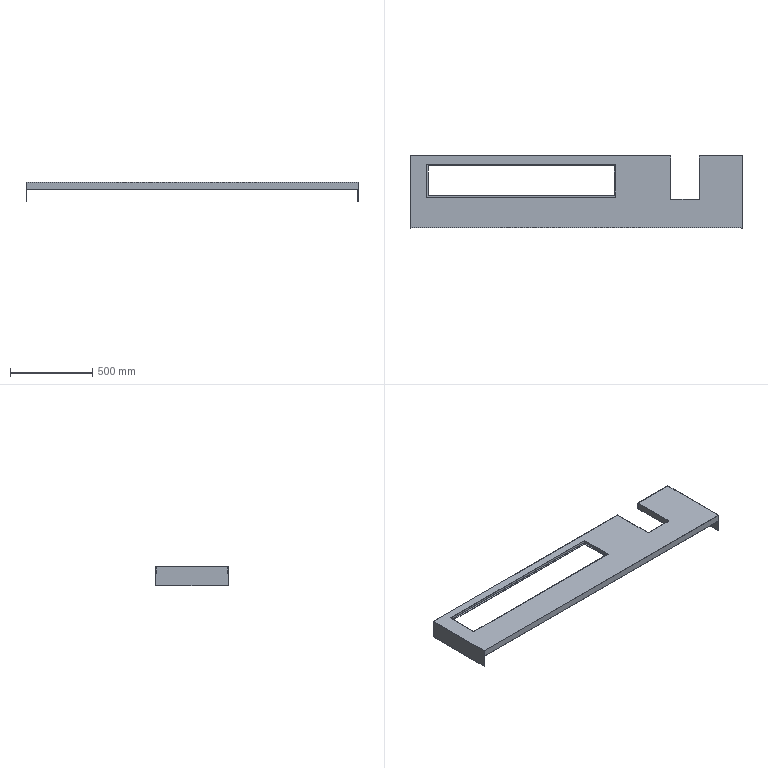Part | SolidWorks | features ICE 7, Extrusion 1 | 1 solid | 36 faces | box 2015 x 437 x 116 mm | volume 1908304 mm3 | plane 36
STEP:
#1=CARTESIAN_POINT('',(100.,387.,-13.));
#2=VERTEX_POINT('',#1);
#3=CARTESIAN_POINT('',(100.,187.,-13.));
#4=VERTEX_POINT('',#3);
#5=CARTESIAN_POINT('',(100.,387.,-13.));
#6=DIRECTION('',(0.,-1.,0.));
#7=VECTOR('',#6,1000.);
#8=LINE('',#5,#7);
#9=EDGE_CURVE('',#2,#4,#8,.T.);
#10=ORIENTED_EDGE('',*,*,#9,.F.);
#11=CARTESIAN_POINT('',(100.,387.,2.));
#12=VERTEX_POINT('',#11);
#13=CARTESIAN_POINT('',(100.,387.,-8.));
#14=DIRECTION('',(0.,0.,1.));
#15=VECTOR('',#14,1000.);
#16=LINE('',#13,#15);
#17=EDGE_CURVE('',#2,#12,#16,.T.);
#18=ORIENTED_EDGE('',*,*,#17,.T.);
#19=CARTESIAN_POINT('',(100.,187.,2.));
#20=VERTEX_POINT('',#19);
#21=CARTESIAN_POINT('',(100.,387.,2.));
#22=DIRECTION('',(0.,-1.,0.));
#23=VECTOR('',#22,1000.);
#24=LINE('',#21,#23);
#25=EDGE_CURVE('',#12,#20,#24,.T.);
#26=ORIENTED_EDGE('',*,*,#25,.T.);
#27=CARTESIAN_POINT('',(100.,187.,-8.));
#28=DIRECTION('',(0.,0.,1.));
#29=VECTOR('',#28,1000.);
#30=LINE('',#27,#29);
#31=EDGE_CURVE('',#4,#20,#30,.T.);
#32=ORIENTED_EDGE('',*,*,#31,.F.);
#33=EDGE_LOOP('',(#10,#18,#26,#32));
#34=FACE_OUTER_BOUND('',#33,.T.);
#35=CARTESIAN_POINT('',(100.,387.,-8.));
#36=DIRECTION('',(-1.,0.,0.));
#37=DIRECTION('',(0.,-1.,0.));
#38=AXIS2_PLACEMENT_3D('',#35,#36,#37);
#39=PLANE('',#38);
#40=ADVANCED_FACE('',(#34),#39,.F.);
#41=CARTESIAN_POINT('',(1250.,387.,-13.));
#42=VERTEX_POINT('',#41);
#43=CARTESIAN_POINT('',(100.,387.,-13.));
#44=DIRECTION('',(-1.,0.,0.));
#45=VECTOR('',#44,1000.);
#46=LINE('',#43,#45);
#47=EDGE_CURVE('',#42,#2,#46,.T.);
#48=ORIENTED_EDGE('',*,*,#47,.F.);
#49=CARTESIAN_POINT('',(1250.,387.,2.));
#50=VERTEX_POINT('',#49);
#51=CARTESIAN_POINT('',(1250.,387.,-8.));
#52=DIRECTION('',(0.,0.,1.));
#53=VECTOR('',#52,1000.);
#54=LINE('',#51,#53);
#55=EDGE_CURVE('',#42,#50,#54,.T.);
#56=ORIENTED_EDGE('',*,*,#55,.T.);
#57=CARTESIAN_POINT('',(100.,387.,2.));
#58=DIRECTION('',(-1.,0.,0.));
#59=VECTOR('',#58,1000.);
#60=LINE('',#57,#59);
#61=EDGE_CURVE('',#50,#12,#60,.T.);
#62=ORIENTED_EDGE('',*,*,#61,.T.);
#63=ORIENTED_EDGE('',*,*,#17,.F.);
#64=EDGE_LOOP('',(#48,#56,#62,#63));
#65=FACE_OUTER_BOUND('',#64,.T.);
#66=CARTESIAN_POINT('',(100.,387.,-8.));
#67=DIRECTION('',(0.,1.,0.));
#68=DIRECTION('',(0.,0.,1.));
#69=AXIS2_PLACEMENT_3D('',#66,#67,#68);
#70=PLANE('',#69);
#71=ADVANCED_FACE('',(#65),#70,.F.);
#72=CARTESIAN_POINT('',(1250.,187.,-13.));
#73=VERTEX_POINT('',#72);
#74=CARTESIAN_POINT('',(1250.,387.,-13.));
#75=DIRECTION('',(0.,1.,0.));
#76=VECTOR('',#75,1000.);
#77=LINE('',#74,#76);
#78=EDGE_CURVE('',#73,#42,#77,.T.);
#79=ORIENTED_EDGE('',*,*,#78,.F.);
#80=CARTESIAN_POINT('',(1250.,187.,2.));
#81=VERTEX_POINT('',#80);
#82=CARTESIAN_POINT('',(1250.,187.,-8.));
#83=DIRECTION('',(0.,0.,1.));
#84=VECTOR('',#83,1000.);
#85=LINE('',#82,#84);
#86=EDGE_CURVE('',#73,#81,#85,.T.);
#87=ORIENTED_EDGE('',*,*,#86,.T.);
#88=CARTESIAN_POINT('',(1250.,387.,2.));
#89=DIRECTION('',(0.,1.,0.));
#90=VECTOR('',#89,1000.);
#91=LINE('',#88,#90);
#92=EDGE_CURVE('',#81,#50,#91,.T.);
#93=ORIENTED_EDGE('',*,*,#92,.T.);
#94=ORIENTED_EDGE('',*,*,#55,.F.);
#95=EDGE_LOOP('',(#79,#87,#93,#94));
#96=FACE_OUTER_BOUND('',#95,.T.);
#97=CARTESIAN_POINT('',(1250.,387.,-8.));
#98=DIRECTION('',(1.,0.,0.));
#99=DIRECTION('',(0.,0.,-1.));
#100=AXIS2_PLACEMENT_3D('',#97,#98,#99);
#101=PLANE('',#100);
#102=ADVANCED_FACE('',(#96),#101,.F.);
#103=CARTESIAN_POINT('',(100.,187.,-13.));
#104=DIRECTION('',(1.,0.,0.));
#105=VECTOR('',#104,1000.);
#106=LINE('',#103,#105);
#107=EDGE_CURVE('',#4,#73,#106,.T.);
#108=ORIENTED_EDGE('',*,*,#107,.F.);
#109=ORIENTED_EDGE('',*,*,#31,.T.);
#110=CARTESIAN_POINT('',(100.,187.,2.));
#111=DIRECTION('',(1.,0.,0.));
#112=VECTOR('',#111,1000.);
#113=LINE('',#110,#112);
#114=EDGE_CURVE('',#20,#81,#113,.T.);
#115=ORIENTED_EDGE('',*,*,#114,.T.);
#116=ORIENTED_EDGE('',*,*,#86,.F.);
#117=EDGE_LOOP('',(#108,#109,#115,#116));
#118=FACE_OUTER_BOUND('',#117,.T.);
#119=CARTESIAN_POINT('',(100.,187.,-8.));
#120=DIRECTION('',(0.,-1.,0.));
#121=DIRECTION('',(0.,0.,-1.));
#122=AXIS2_PLACEMENT_3D('',#119,#120,#121);
#123=PLANE('',#122);
#124=ADVANCED_FACE('',(#118),#123,.F.);
#125=CARTESIAN_POINT('',(2013.,2.,0.));
#126=VERTEX_POINT('',#125);
#127=CARTESIAN_POINT('',(2013.,435.,0.));
#128=VERTEX_POINT('',#127);
#129=CARTESIAN_POINT('',(2013.,0.,0.));
#130=DIRECTION('',(0.,1.,0.));
#131=VECTOR('',#130,1000.);
#132=LINE('',#129,#131);
#133=EDGE_CURVE('',#126,#128,#132,.T.);
#134=ORIENTED_EDGE('',*,*,#133,.F.);
#135=CARTESIAN_POINT('',(2.,2.,0.));
#136=VERTEX_POINT('',#135);
#137=CARTESIAN_POINT('',(0.,2.,0.));
#138=DIRECTION('',(-1.,0.,0.));
#139=VECTOR('',#138,1000.);
#140=LINE('',#137,#139);
#141=EDGE_CURVE('',#126,#136,#140,.T.);
#142=ORIENTED_EDGE('',*,*,#141,.T.);
#143=CARTESIAN_POINT('',(2.,435.,0.));
#144=VERTEX_POINT('',#143);
#145=CARTESIAN_POINT('',(2.,437.,0.));
#146=DIRECTION('',(0.,-1.,0.));
#147=VECTOR('',#146,1000.);
#148=LINE('',#145,#147);
#149=EDGE_CURVE('',#144,#136,#148,.T.);
#150=ORIENTED_EDGE('',*,*,#149,.F.);
#151=CARTESIAN_POINT('',(1580.,435.,0.));
#152=VERTEX_POINT('',#151);
#153=CARTESIAN_POINT('',(1580.,435.,0.));
#154=DIRECTION('',(-1.,0.,0.));
#155=VECTOR('',#154,1000.);
#156=LINE('',#153,#155);
#157=EDGE_CURVE('',#152,#144,#156,.T.);
#158=ORIENTED_EDGE('',*,*,#157,.F.);
#159=CARTESIAN_POINT('',(1580.,171.,0.));
#160=VERTEX_POINT('',#159);
#161=CARTESIAN_POINT('',(1580.,171.,0.));
#162=DIRECTION('',(0.,1.,0.));
#163=VECTOR('',#162,1000.);
#164=LINE('',#161,#163);
#165=EDGE_CURVE('',#160,#152,#164,.T.);
#166=ORIENTED_EDGE('',*,*,#165,.F.);
#167=CARTESIAN_POINT('',(1759.,171.,0.));
#168=VERTEX_POINT('',#167);
#169=CARTESIAN_POINT('',(1759.,171.,0.));
#170=DIRECTION('',(-1.,0.,0.));
#171=VECTOR('',#170,1000.);
#172=LINE('',#169,#171);
#173=EDGE_CURVE('',#168,#160,#172,.T.);
#174=ORIENTED_EDGE('',*,*,#173,.F.);
#175=CARTESIAN_POINT('',(1759.,435.,0.));
#176=VERTEX_POINT('',#175);
#177=CARTESIAN_POINT('',(1759.,435.,0.));
#178=DIRECTION('',(0.,-1.,0.));
#179=VECTOR('',#178,1000.);
#180=LINE('',#177,#179);
#181=EDGE_CURVE('',#176,#168,#180,.T.);
#182=ORIENTED_EDGE('',*,*,#181,.F.);
#183=CARTESIAN_POINT('',(2013.,435.,0.));
#184=DIRECTION('',(-1.,0.,0.));
#185=VECTOR('',#184,1000.);
#186=LINE('',#183,#185);
#187=EDGE_CURVE('',#128,#176,#186,.T.);
#188=ORIENTED_EDGE('',*,*,#187,.F.);
#189=EDGE_LOOP('',(#134,#142,#150,#158,#166,#174,#182,#188));
#190=FACE_OUTER_BOUND('',#189,.T.);
#191=CARTESIAN_POINT('',(1252.,389.,0.));
#192=VERTEX_POINT('',#191);
#193=CARTESIAN_POINT('',(1252.,185.,0.));
#194=VERTEX_POINT('',#193);
#195=CARTESIAN_POINT('',(1252.,389.,0.));
#196=DIRECTION('',(0.,-1.,0.));
#197=VECTOR('',#196,1000.);
#198=LINE('',#195,#197);
#199=EDGE_CURVE('',#192,#194,#198,.T.);
#200=ORIENTED_EDGE('',*,*,#199,.F.);
#201=CARTESIAN_POINT('',(98.,389.,0.));
#202=VERTEX_POINT('',#201);
#203=CARTESIAN_POINT('',(98.,389.,0.));
#204=DIRECTION('',(1.,0.,0.));
#205=VECTOR('',#204,1000.);
#206=LINE('',#203,#205);
#207=EDGE_CURVE('',#202,#192,#206,.T.);
#208=ORIENTED_EDGE('',*,*,#207,.F.);
#209=CARTESIAN_POINT('',(98.,185.,0.));
#210=VERTEX_POINT('',#209);
#211=CARTESIAN_POINT('',(98.,185.,0.));
#212=DIRECTION('',(0.,1.,0.));
#213=VECTOR('',#212,1000.);
#214=LINE('',#211,#213);
#215=EDGE_CURVE('',#210,#202,#214,.T.);
#216=ORIENTED_EDGE('',*,*,#215,.F.);
#217=CARTESIAN_POINT('',(1252.,185.,0.));
#218=DIRECTION('',(-1.,0.,0.));
#219=VECTOR('',#218,1000.);
#220=LINE('',#217,#219);
#221=EDGE_CURVE('',#194,#210,#220,.T.);
#222=ORIENTED_EDGE('',*,*,#221,.F.);
#223=EDGE_LOOP('',(#200,#208,#216,#222));
#224=FACE_BOUND('',#223,.T.);
#225=CARTESIAN_POINT('',(0.,437.,0.));
#226=DIRECTION('',(0.,0.,-1.));
#227=DIRECTION('',(-1.,0.,0.));
#228=AXIS2_PLACEMENT_3D('',#225,#226,#227);
#229=PLANE('',#228);
#230=ADVANCED_FACE('',(#190,#224),#229,.T.);
#231=CARTESIAN_POINT('',(2013.,0.,-114.));
#232=VERTEX_POINT('',#231);
#233=CARTESIAN_POINT('',(2013.,0.,-40.468));
#234=VERTEX_POINT('',#233);
#235=CARTESIAN_POINT('',(2013.,0.,-114.));
#236=DIRECTION('',(0.,0.,1.));
#237=VECTOR('',#236,1000.);
#238=LINE('',#235,#237);
#239=EDGE_CURVE('',#232,#234,#238,.T.);
#240=ORIENTED_EDGE('',*,*,#239,.T.);
#241=CARTESIAN_POINT('',(2013.,2.,-40.468));
#242=VERTEX_POINT('',#241);
#243=CARTESIAN_POINT('',(2013.,0.,-40.468));
#244=DIRECTION('',(0.,1.,0.));
#245=VECTOR('',#244,1000.);
#246=LINE('',#243,#245);
#247=EDGE_CURVE('',#234,#242,#246,.T.);
#248=ORIENTED_EDGE('',*,*,#247,.T.);
#249=CARTESIAN_POINT('',(2013.,2.,-114.));
#250=DIRECTION('',(0.,0.,-1.));
#251=VECTOR('',#250,1000.);
#252=LINE('',#249,#251);
#253=EDGE_CURVE('',#126,#242,#252,.T.);
#254=ORIENTED_EDGE('',*,*,#253,.F.);
#255=ORIENTED_EDGE('',*,*,#133,.T.);
#256=CARTESIAN_POINT('',(2013.,435.,-40.));
#257=VERTEX_POINT('',#256);
#258=CARTESIAN_POINT('',(2013.,435.,-40.));
#259=DIRECTION('',(0.,0.,1.));
#260=VECTOR('',#259,1000.);
#261=LINE('',#258,#260);
#262=EDGE_CURVE('',#257,#128,#261,.T.);
#263=ORIENTED_EDGE('',*,*,#262,.F.);
#264=CARTESIAN_POINT('',(2013.,437.,-40.));
#265=VERTEX_POINT('',#264);
#266=CARTESIAN_POINT('',(2013.,437.,-40.));
#267=DIRECTION('',(0.,-1.,0.));
#268=VECTOR('',#267,1000.);
#269=LINE('',#266,#268);
#270=EDGE_CURVE('',#265,#257,#269,.T.);
#271=ORIENTED_EDGE('',*,*,#270,.F.);
#272=CARTESIAN_POINT('',(2013.,437.,-114.));
#273=VERTEX_POINT('',#272);
#274=CARTESIAN_POINT('',(2013.,437.,-114.));
#275=DIRECTION('',(0.,0.,1.));
#276=VECTOR('',#275,1000.);
#277=LINE('',#274,#276);
#278=EDGE_CURVE('',#273,#265,#277,.T.);
#279=ORIENTED_EDGE('',*,*,#278,.F.);
#280=CARTESIAN_POINT('',(2013.,0.,-114.));
#281=DIRECTION('',(0.,1.,0.));
#282=VECTOR('',#281,1000.);
#283=LINE('',#280,#282);
#284=EDGE_CURVE('',#232,#273,#283,.T.);
#285=ORIENTED_EDGE('',*,*,#284,.F.);
#286=EDGE_LOOP('',(#240,#248,#254,#255,#263,#271,#279,#285));
#287=FACE_OUTER_BOUND('',#286,.T.);
#288=CARTESIAN_POINT('',(2013.,0.,-114.));
#289=DIRECTION('',(1.,0.,0.));
#290=DIRECTION('',(0.,0.,-1.));
#291=AXIS2_PLACEMENT_3D('',#288,#289,#290);
#292=PLANE('',#291);
#293=ADVANCED_FACE('',(#287),#292,.F.);
#294=CARTESIAN_POINT('',(2.,2.,-40.468));
#295=VERTEX_POINT('',#294);
#296=CARTESIAN_POINT('',(2.,2.,-114.));
#297=DIRECTION('',(0.,0.,1.));
#298=VECTOR('',#297,1000.);
#299=LINE('',#296,#298);
#300=EDGE_CURVE('',#295,#136,#299,.T.);
#301=ORIENTED_EDGE('',*,*,#300,.F.);
#302=CARTESIAN_POINT('',(2.,0.,-40.468));
#303=VERTEX_POINT('',#302);
#304=CARTESIAN_POINT('',(2.,437.,-40.468));
#305=DIRECTION('',(0.,-1.,0.));
#306=VECTOR('',#305,1000.);
#307=LINE('',#304,#306);
#308=EDGE_CURVE('',#295,#303,#307,.T.);
#309=ORIENTED_EDGE('',*,*,#308,.T.);
#310=CARTESIAN_POINT('',(2.,0.,-114.));
#311=VERTEX_POINT('',#310);
#312=CARTESIAN_POINT('',(2.,0.,-114.));
#313=DIRECTION('',(0.,0.,1.));
#314=VECTOR('',#313,1000.);
#315=LINE('',#312,#314);
#316=EDGE_CURVE('',#311,#303,#315,.T.);
#317=ORIENTED_EDGE('',*,*,#316,.F.);
#318=CARTESIAN_POINT('',(2.,437.,-114.));
#319=VERTEX_POINT('',#318);
#320=CARTESIAN_POINT('',(2.,437.,-114.));
#321=DIRECTION('',(0.,-1.,0.));
#322=VECTOR('',#321,1000.);
#323=LINE('',#320,#322);
#324=EDGE_CURVE('',#319,#311,#323,.T.);
#325=ORIENTED_EDGE('',*,*,#324,.F.);
#326=CARTESIAN_POINT('',(2.,437.,-40.));
#327=VERTEX_POINT('',#326);
#328=CARTESIAN_POINT('',(2.,437.,-114.));
#329=DIRECTION('',(0.,0.,1.));
#330=VECTOR('',#329,1000.);
#331=LINE('',#328,#330);
#332=EDGE_CURVE('',#319,#327,#331,.T.);
#333=ORIENTED_EDGE('',*,*,#332,.T.);
#334=CARTESIAN_POINT('',(2.,435.,-40.));
#335=VERTEX_POINT('',#334);
#336=CARTESIAN_POINT('',(2.,437.,-40.));
#337=DIRECTION('',(0.,1.,0.));
#338=VECTOR('',#337,1000.);
#339=LINE('',#336,#338);
#340=EDGE_CURVE('',#335,#327,#339,.T.);
#341=ORIENTED_EDGE('',*,*,#340,.F.);
#342=CARTESIAN_POINT('',(2.,435.,-40.));
#343=DIRECTION('',(0.,0.,1.));
#344=VECTOR('',#343,1000.);
#345=LINE('',#342,#344);
#346=EDGE_CURVE('',#335,#144,#345,.T.);
#347=ORIENTED_EDGE('',*,*,#346,.T.);
#348=ORIENTED_EDGE('',*,*,#149,.T.);
#349=EDGE_LOOP('',(#301,#309,#317,#325,#333,#341,#347,#348));
#350=FACE_OUTER_BOUND('',#349,.T.);
#351=CARTESIAN_POINT('',(2.,437.,-114.));
#352=DIRECTION('',(-1.,0.,0.));
#353=DIRECTION('',(0.,-1.,0.));
#354=AXIS2_PLACEMENT_3D('',#351,#352,#353);
#355=PLANE('',#354);
#356=ADVANCED_FACE('',(#350),#355,.F.);
#357=CARTESIAN_POINT('',(0.,0.,-114.));
#358=VERTEX_POINT('',#357);
#359=CARTESIAN_POINT('',(0.,437.,-114.));
#360=VERTEX_POINT('',#359);
#361=CARTESIAN_POINT('',(0.,437.,-114.));
#362=DIRECTION('',(0.,1.,0.));
#363=VECTOR('',#362,1000.);
#364=LINE('',#361,#363);
#365=EDGE_CURVE('',#358,#360,#364,.T.);
#366=ORIENTED_EDGE('',*,*,#365,.F.);
#367=CARTESIAN_POINT('',(0.,0.,2.));
#368=VERTEX_POINT('',#367);
#369=CARTESIAN_POINT('',(0.,0.,2.));
#370=DIRECTION('',(0.,0.,-1.));
#371=VECTOR('',#370,1000.);
#372=LINE('',#369,#371);
#373=EDGE_CURVE('',#368,#358,#372,.T.);
#374=ORIENTED_EDGE('',*,*,#373,.F.);
#375=CARTESIAN_POINT('',(0.,437.,2.));
#376=VERTEX_POINT('',#375);
#377=CARTESIAN_POINT('',(0.,0.,2.));
#378=DIRECTION('',(0.,-1.,0.));
#379=VECTOR('',#378,1000.);
#380=LINE('',#377,#379);
#381=EDGE_CURVE('',#376,#368,#380,.T.);
#382=ORIENTED_EDGE('',*,*,#381,.F.);
#383=CARTESIAN_POINT('',(0.,437.,2.));
#384=DIRECTION('',(0.,0.,-1.));
#385=VECTOR('',#384,1000.);
#386=LINE('',#383,#385);
#387=EDGE_CURVE('',#376,#360,#386,.T.);
#388=ORIENTED_EDGE('',*,*,#387,.T.);
#389=EDGE_LOOP('',(#366,#374,#382,#388));
#390=FACE_OUTER_BOUND('',#389,.T.);
#391=CARTESIAN_POINT('',(0.,0.,2.));
#392=DIRECTION('',(1.,0.,0.));
#393=DIRECTION('',(0.,0.,-1.));
#394=AXIS2_PLACEMENT_3D('',#391,#392,#393);
#395=PLANE('',#394);
#396=ADVANCED_FACE('',(#390),#395,.F.);
#397=CARTESIAN_POINT('',(0.,0.,-40.468));
#398=DIRECTION('',(1.,0.,0.));
#399=VECTOR('',#398,1000.);
#400=LINE('',#397,#399);
#401=EDGE_CURVE('',#303,#234,#400,.T.);
#402=ORIENTED_EDGE('',*,*,#401,.T.);
#403=ORIENTED_EDGE('',*,*,#239,.F.);
#404=CARTESIAN_POINT('',(2015.,0.,-114.));
#405=VERTEX_POINT('',#404);
#406=CARTESIAN_POINT('',(2015.,0.,-114.));
#407=DIRECTION('',(-1.,0.,0.));
#408=VECTOR('',#407,1000.);
#409=LINE('',#406,#408);
#410=EDGE_CURVE('',#405,#232,#409,.T.);
#411=ORIENTED_EDGE('',*,*,#410,.F.);
#412=CARTESIAN_POINT('',(2015.,0.,2.));
#413=VERTEX_POINT('',#412);
#414=CARTESIAN_POINT('',(2015.,0.,2.));
#415=DIRECTION('',(0.,0.,-1.));
#416=VECTOR('',#415,1000.);
#417=LINE('',#414,#416);
#418=EDGE_CURVE('',#413,#405,#417,.T.);
#419=ORIENTED_EDGE('',*,*,#418,.F.);
#420=CARTESIAN_POINT('',(0.,0.,2.));
#421=DIRECTION('',(1.,0.,0.));
#422=VECTOR('',#421,1000.);
#423=LINE('',#420,#422);
#424=EDGE_CURVE('',#368,#413,#423,.T.);
#425=ORIENTED_EDGE('',*,*,#424,.F.);
#426=ORIENTED_EDGE('',*,*,#373,.T.);
#427=CARTESIAN_POINT('',(0.,0.,-114.));
#428=DIRECTION('',(-1.,0.,0.));
#429=VECTOR('',#428,1000.);
#430=LINE('',#427,#429);
#431=EDGE_CURVE('',#311,#358,#430,.T.);
#432=ORIENTED_EDGE('',*,*,#431,.F.);
#433=ORIENTED_EDGE('',*,*,#316,.T.);
#434=EDGE_LOOP('',(#402,#403,#411,#419,#425,#426,#432,#433));
#435=FACE_OUTER_BOUND('',#434,.T.);
#436=CARTESIAN_POINT('',(0.,0.,2.));
#437=DIRECTION('',(0.,1.,0.));
#438=DIRECTION('',(0.,0.,1.));
#439=AXIS2_PLACEMENT_3D('',#436,#437,#438);
#440=PLANE('',#439);
#441=ADVANCED_FACE('',(#435),#440,.F.);
#442=ORIENTED_EDGE('',*,*,#418,.T.);
#443=CARTESIAN_POINT('',(2015.,437.,-114.));
#444=VERTEX_POINT('',#443);
#445=CARTESIAN_POINT('',(2015.,437.,-114.));
#446=DIRECTION('',(0.,-1.,0.));
#447=VECTOR('',#446,1000.);
#448=LINE('',#445,#447);
#449=EDGE_CURVE('',#444,#405,#448,.T.);
#450=ORIENTED_EDGE('',*,*,#449,.F.);
#451=CARTESIAN_POINT('',(2015.,437.,2.));
#452=VERTEX_POINT('',#451);
#453=CARTESIAN_POINT('',(2015.,437.,2.));
#454=DIRECTION('',(0.,0.,-1.));
#455=VECTOR('',#454,1000.);
#456=LINE('',#453,#455);
#457=EDGE_CURVE('',#452,#444,#456,.T.);
#458=ORIENTED_EDGE('',*,*,#457,.F.);
#459=CARTESIAN_POINT('',(2015.,0.,2.));
#460=DIRECTION('',(0.,1.,0.));
#461=VECTOR('',#460,1000.);
#462=LINE('',#459,#461);
#463=EDGE_CURVE('',#413,#452,#462,.T.);
#464=ORIENTED_EDGE('',*,*,#463,.F.);
#465=EDGE_LOOP('',(#442,#450,#458,#464));
#466=FACE_OUTER_BOUND('',#465,.T.);
#467=CARTESIAN_POINT('',(2015.,0.,2.));
#468=DIRECTION('',(-1.,0.,0.));
#469=DIRECTION('',(0.,0.,1.));
#470=AXIS2_PLACEMENT_3D('',#467,#468,#469);
#471=PLANE('',#470);
#472=ADVANCED_FACE('',(#466),#471,.F.);
#473=CARTESIAN_POINT('',(1757.,437.,-40.));
#474=VERTEX_POINT('',#473);
#475=CARTESIAN_POINT('',(2013.,437.,-40.));
#476=DIRECTION('',(1.,0.,0.));
#477=VECTOR('',#476,1000.);
#478=LINE('',#475,#477);
#479=EDGE_CURVE('',#474,#265,#478,.T.);
#480=ORIENTED_EDGE('',*,*,#479,.F.);
#481=CARTESIAN_POINT('',(1757.,437.,2.));
#482=VERTEX_POINT('',#481);
#483=CARTESIAN_POINT('',(1757.,437.,2.));
#484=DIRECTION('',(0.,0.,-1.));
#485=VECTOR('',#484,1000.);
#486=LINE('',#483,#485);
#487=EDGE_CURVE('',#482,#474,#486,.T.);
#488=ORIENTED_EDGE('',*,*,#487,.F.);
#489=CARTESIAN_POINT('',(1757.,437.,2.));
#490=DIRECTION('',(-1.,0.,0.));
#491=VECTOR('',#490,1000.);
#492=LINE('',#489,#491);
#493=EDGE_CURVE('',#452,#482,#492,.T.);
#494=ORIENTED_EDGE('',*,*,#493,.F.);
#495=ORIENTED_EDGE('',*,*,#457,.T.);
#496=CARTESIAN_POINT('',(2013.,437.,-114.));
#497=DIRECTION('',(1.,0.,0.));
#498=VECTOR('',#497,1000.);
#499=LINE('',#496,#498);
#500=EDGE_CURVE('',#273,#444,#499,.T.);
#501=ORIENTED_EDGE('',*,*,#500,.F.);
#502=ORIENTED_EDGE('',*,*,#278,.T.);
#503=EDGE_LOOP('',(#480,#488,#494,#495,#501,#502));
#504=FACE_OUTER_BOUND('',#503,.T.);
#505=CARTESIAN_POINT('',(1757.,437.,2.));
#506=DIRECTION('',(0.,-1.,0.));
#507=DIRECTION('',(0.,0.,-1.));
#508=AXIS2_PLACEMENT_3D('',#505,#506,#507);
#509=PLANE('',#508);
#510=ADVANCED_FACE('',(#504),#509,.F.);
#511=ORIENTED_EDGE('',*,*,#487,.T.);
#512=CARTESIAN_POINT('',(1757.,173.,-40.));
#513=VERTEX_POINT('',#512);
#514=CARTESIAN_POINT('',(1757.,437.,-40.));
#515=DIRECTION('',(0.,1.,0.));
#516=VECTOR('',#515,1000.);
#517=LINE('',#514,#516);
#518=EDGE_CURVE('',#513,#474,#517,.T.);
#519=ORIENTED_EDGE('',*,*,#518,.F.);
#520=CARTESIAN_POINT('',(1757.,173.,2.));
#521=VERTEX_POINT('',#520);
#522=CARTESIAN_POINT('',(1757.,173.,2.));
#523=DIRECTION('',(0.,0.,-1.));
#524=VECTOR('',#523,1000.);
#525=LINE('',#522,#524);
#526=EDGE_CURVE('',#521,#513,#525,.T.);
#527=ORIENTED_EDGE('',*,*,#526,.F.);
#528=CARTESIAN_POINT('',(1757.,437.,2.));
#529=DIRECTION('',(0.,-1.,0.));
#530=VECTOR('',#529,1000.);
#531=LINE('',#528,#530);
#532=EDGE_CURVE('',#482,#521,#531,.T.);
#533=ORIENTED_EDGE('',*,*,#532,.F.);
#534=EDGE_LOOP('',(#511,#519,#527,#533));
#535=FACE_OUTER_BOUND('',#534,.T.);
#536=CARTESIAN_POINT('',(1757.,437.,2.));
#537=DIRECTION('',(1.,0.,0.));
#538=DIRECTION('',(0.,0.,-1.));
#539=AXIS2_PLACEMENT_3D('',#536,#537,#538);
#540=PLANE('',#539);
#541=ADVANCED_FACE('',(#535),#540,.F.);
#542=ORIENTED_EDGE('',*,*,#526,.T.);
#543=CARTESIAN_POINT('',(1582.,173.,-40.));
#544=VERTEX_POINT('',#543);
#545=CARTESIAN_POINT('',(1757.,173.,-40.));
#546=DIRECTION('',(1.,0.,0.));
#547=VECTOR('',#546,1000.);
#548=LINE('',#545,#547);
#549=EDGE_CURVE('',#544,#513,#548,.T.);
#550=ORIENTED_EDGE('',*,*,#549,.F.);
#551=CARTESIAN_POINT('',(1582.,173.,2.));
#552=VERTEX_POINT('',#551);
#553=CARTESIAN_POINT('',(1582.,173.,2.));
#554=DIRECTION('',(0.,0.,-1.));
#555=VECTOR('',#554,1000.);
#556=LINE('',#553,#555);
#557=EDGE_CURVE('',#552,#544,#556,.T.);
#558=ORIENTED_EDGE('',*,*,#557,.F.);
#559=CARTESIAN_POINT('',(1582.,173.,2.));
#560=DIRECTION('',(-1.,0.,0.));
#561=VECTOR('',#560,1000.);
#562=LINE('',#559,#561);
#563=EDGE_CURVE('',#521,#552,#562,.T.);
#564=ORIENTED_EDGE('',*,*,#563,.F.);
#565=EDGE_LOOP('',(#542,#550,#558,#564));
#566=FACE_OUTER_BOUND('',#565,.T.);
#567=CARTESIAN_POINT('',(1582.,173.,2.));
#568=DIRECTION('',(0.,-1.,0.));
#569=DIRECTION('',(1.,0.,0.));
#570=AXIS2_PLACEMENT_3D('',#567,#568,#569);
#571=PLANE('',#570);
#572=ADVANCED_FACE('',(#566),#571,.F.);
#573=ORIENTED_EDGE('',*,*,#557,.T.);
#574=CARTESIAN_POINT('',(1582.,437.,-40.));
#575=VERTEX_POINT('',#574);
#576=CARTESIAN_POINT('',(1582.,173.,-40.));
#577=DIRECTION('',(0.,-1.,0.));
#578=VECTOR('',#577,1000.);
#579=LINE('',#576,#578);
#580=EDGE_CURVE('',#575,#544,#579,.T.);
#581=ORIENTED_EDGE('',*,*,#580,.F.);
#582=CARTESIAN_POINT('',(1582.,437.,2.));
#583=VERTEX_POINT('',#582);
#584=CARTESIAN_POINT('',(1582.,437.,2.));
#585=DIRECTION('',(0.,0.,-1.));
#586=VECTOR('',#585,1000.);
#587=LINE('',#584,#586);
#588=EDGE_CURVE('',#583,#575,#587,.T.);
#589=ORIENTED_EDGE('',*,*,#588,.F.);
#590=CARTESIAN_POINT('',(1582.,437.,2.));
#591=DIRECTION('',(0.,1.,0.));
#592=VECTOR('',#591,1000.);
#593=LINE('',#590,#592);
#594=EDGE_CURVE('',#552,#583,#593,.T.);
#595=ORIENTED_EDGE('',*,*,#594,.F.);
#596=EDGE_LOOP('',(#573,#581,#589,#595));
#597=FACE_OUTER_BOUND('',#596,.T.);
#598=CARTESIAN_POINT('',(1582.,437.,2.));
#599=DIRECTION('',(-1.,0.,0.));
#600=DIRECTION('',(0.,0.,1.));
#601=AXIS2_PLACEMENT_3D('',#598,#599,#600);
#602=PLANE('',#601);
#603=ADVANCED_FACE('',(#597),#602,.F.);
#604=ORIENTED_EDGE('',*,*,#588,.T.);
#605=CARTESIAN_POINT('',(1582.,437.,-40.));
#606=DIRECTION('',(1.,0.,0.));
#607=VECTOR('',#606,1000.);
#608=LINE('',#605,#607);
#609=EDGE_CURVE('',#327,#575,#608,.T.);
#610=ORIENTED_EDGE('',*,*,#609,.F.);
#611=ORIENTED_EDGE('',*,*,#332,.F.);
#612=CARTESIAN_POINT('',(0.,437.,-114.));
#613=DIRECTION('',(1.,0.,0.));
#614=VECTOR('',#613,1000.);
#615=LINE('',#612,#614);
#616=EDGE_CURVE('',#360,#319,#615,.T.);
#617=ORIENTED_EDGE('',*,*,#616,.F.);
#618=ORIENTED_EDGE('',*,*,#387,.F.);
#619=CARTESIAN_POINT('',(0.,437.,2.));
#620=DIRECTION('',(-1.,0.,0.));
#621=VECTOR('',#620,1000.);
#622=LINE('',#619,#621);
#623=EDGE_CURVE('',#583,#376,#622,.T.);
#624=ORIENTED_EDGE('',*,*,#623,.F.);
#625=EDGE_LOOP('',(#604,#610,#611,#617,#618,#624));
#626=FACE_OUTER_BOUND('',#625,.T.);
#627=CARTESIAN_POINT('',(0.,437.,2.));
#628=DIRECTION('',(0.,-1.,0.));
#629=DIRECTION('',(0.,0.,-1.));
#630=AXIS2_PLACEMENT_3D('',#627,#628,#629);
#631=PLANE('',#630);
#632=ADVANCED_FACE('',(#626),#631,.F.);
#633=ORIENTED_EDGE('',*,*,#463,.T.);
#634=ORIENTED_EDGE('',*,*,#493,.T.);
#635=ORIENTED_EDGE('',*,*,#532,.T.);
#636=ORIENTED_EDGE('',*,*,#563,.T.);
#637=ORIENTED_EDGE('',*,*,#594,.T.);
#638=ORIENTED_EDGE('',*,*,#623,.T.);
#639=ORIENTED_EDGE('',*,*,#381,.T.);
#640=ORIENTED_EDGE('',*,*,#424,.T.);
#641=EDGE_LOOP('',(#633,#634,#635,#636,#637,#638,#639,#640));
#642=FACE_OUTER_BOUND('',#641,.T.);
#643=ORIENTED_EDGE('',*,*,#114,.F.);
#644=ORIENTED_EDGE('',*,*,#25,.F.);
#645=ORIENTED_EDGE('',*,*,#61,.F.);
#646=ORIENTED_EDGE('',*,*,#92,.F.);
#647=EDGE_LOOP('',(#643,#644,#645,#646));
#648=FACE_BOUND('',#647,.T.);
#649=CARTESIAN_POINT('',(0.,437.,2.));
#650=DIRECTION('',(0.,0.,-1.));
#651=DIRECTION('',(-1.,0.,0.));
#652=AXIS2_PLACEMENT_3D('',#649,#650,#651);
#653=PLANE('',#652);
#654=ADVANCED_FACE('',(#642,#648),#653,.F.);
#655=ORIENTED_EDGE('',*,*,#449,.T.);
#656=ORIENTED_EDGE('',*,*,#410,.T.);
#657=ORIENTED_EDGE('',*,*,#284,.T.);
#658=ORIENTED_EDGE('',*,*,#500,.T.);
#659=EDGE_LOOP('',(#655,#656,#657,#658));
#660=FACE_OUTER_BOUND('',#659,.T.);
#661=CARTESIAN_POINT('',(2015.,0.,-114.));
#662=DIRECTION('',(0.,0.,-1.));
#663=DIRECTION('',(-1.,0.,0.));
#664=AXIS2_PLACEMENT_3D('',#661,#662,#663);
#665=PLANE('',#664);
#666=ADVANCED_FACE('',(#660),#665,.T.);
#667=ORIENTED_EDGE('',*,*,#365,.T.);
#668=ORIENTED_EDGE('',*,*,#616,.T.);
#669=ORIENTED_EDGE('',*,*,#324,.T.);
#670=ORIENTED_EDGE('',*,*,#431,.T.);
#671=EDGE_LOOP('',(#667,#668,#669,#670));
#672=FACE_OUTER_BOUND('',#671,.T.);
#673=CARTESIAN_POINT('',(0.,0.,-114.));
#674=DIRECTION('',(0.,0.,1.));
#675=DIRECTION('',(1.,0.,0.));
#676=AXIS2_PLACEMENT_3D('',#673,#674,#675);
#677=PLANE('',#676);
#678=ADVANCED_FACE('',(#672),#677,.F.);
#679=ORIENTED_EDGE('',*,*,#187,.T.);
#680=CARTESIAN_POINT('',(1759.,435.,-40.));
#681=VERTEX_POINT('',#680);
#682=CARTESIAN_POINT('',(1759.,435.,-40.));
#683=DIRECTION('',(0.,0.,1.));
#684=VECTOR('',#683,1000.);
#685=LINE('',#682,#684);
#686=EDGE_CURVE('',#681,#176,#685,.T.);
#687=ORIENTED_EDGE('',*,*,#686,.F.);
#688=CARTESIAN_POINT('',(2013.,435.,-40.));
#689=DIRECTION('',(-1.,0.,0.));
#690=VECTOR('',#689,1000.);
#691=LINE('',#688,#690);
#692=EDGE_CURVE('',#257,#681,#691,.T.);
#693=ORIENTED_EDGE('',*,*,#692,.F.);
#694=ORIENTED_EDGE('',*,*,#262,.T.);
#695=EDGE_LOOP('',(#679,#687,#693,#694));
#696=FACE_OUTER_BOUND('',#695,.T.);
#697=CARTESIAN_POINT('',(2013.,435.,-40.));
#698=DIRECTION('',(0.,1.,0.));
#699=DIRECTION('',(0.,0.,1.));
#700=AXIS2_PLACEMENT_3D('',#697,#698,#699);
#701=PLANE('',#700);
#702=ADVANCED_FACE('',(#696),#701,.F.);
#703=ORIENTED_EDGE('',*,*,#181,.T.);
#704=CARTESIAN_POINT('',(1759.,171.,-40.));
#705=VERTEX_POINT('',#704);
#706=CARTESIAN_POINT('',(1759.,171.,-40.));
#707=DIRECTION('',(0.,0.,1.));
#708=VECTOR('',#707,1000.);
#709=LINE('',#706,#708);
#710=EDGE_CURVE('',#705,#168,#709,.T.);
#711=ORIENTED_EDGE('',*,*,#710,.F.);
#712=CARTESIAN_POINT('',(1759.,435.,-40.));
#713=DIRECTION('',(0.,-1.,0.));
#714=VECTOR('',#713,1000.);
#715=LINE('',#712,#714);
#716=EDGE_CURVE('',#681,#705,#715,.T.);
#717=ORIENTED_EDGE('',*,*,#716,.F.);
#718=ORIENTED_EDGE('',*,*,#686,.T.);
#719=EDGE_LOOP('',(#703,#711,#717,#718));
#720=FACE_OUTER_BOUND('',#719,.T.);
#721=CARTESIAN_POINT('',(1759.,435.,-40.));
#722=DIRECTION('',(-1.,0.,0.));
#723=DIRECTION('',(0.,0.,1.));
#724=AXIS2_PLACEMENT_3D('',#721,#722,#723);
#725=PLANE('',#724);
#726=ADVANCED_FACE('',(#720),#725,.F.);
#727=ORIENTED_EDGE('',*,*,#173,.T.);
#728=CARTESIAN_POINT('',(1580.,171.,-40.));
#729=VERTEX_POINT('',#728);
#730=CARTESIAN_POINT('',(1580.,171.,-40.));
#731=DIRECTION('',(0.,0.,1.));
#732=VECTOR('',#731,1000.);
#733=LINE('',#730,#732);
#734=EDGE_CURVE('',#729,#160,#733,.T.);
#735=ORIENTED_EDGE('',*,*,#734,.F.);
#736=CARTESIAN_POINT('',(1759.,171.,-40.));
#737=DIRECTION('',(-1.,0.,0.));
#738=VECTOR('',#737,1000.);
#739=LINE('',#736,#738);
#740=EDGE_CURVE('',#705,#729,#739,.T.);
#741=ORIENTED_EDGE('',*,*,#740,.F.);
#742=ORIENTED_EDGE('',*,*,#710,.T.);
#743=EDGE_LOOP('',(#727,#735,#741,#742));
#744=FACE_OUTER_BOUND('',#743,.T.);
#745=CARTESIAN_POINT('',(1759.,171.,-40.));
#746=DIRECTION('',(0.,1.,0.));
#747=DIRECTION('',(0.,0.,1.));
#748=AXIS2_PLACEMENT_3D('',#745,#746,#747);
#749=PLANE('',#748);
#750=ADVANCED_FACE('',(#744),#749,.F.);
#751=ORIENTED_EDGE('',*,*,#165,.T.);
#752=CARTESIAN_POINT('',(1580.,435.,-40.));
#753=VERTEX_POINT('',#752);
#754=CARTESIAN_POINT('',(1580.,435.,-40.));
#755=DIRECTION('',(0.,0.,1.));
#756=VECTOR('',#755,1000.);
#757=LINE('',#754,#756);
#758=EDGE_CURVE('',#753,#152,#757,.T.);
#759=ORIENTED_EDGE('',*,*,#758,.F.);
#760=CARTESIAN_POINT('',(1580.,171.,-40.));
#761=DIRECTION('',(0.,1.,0.));
#762=VECTOR('',#761,1000.);
#763=LINE('',#760,#762);
#764=EDGE_CURVE('',#729,#753,#763,.T.);
#765=ORIENTED_EDGE('',*,*,#764,.F.);
#766=ORIENTED_EDGE('',*,*,#734,.T.);
#767=EDGE_LOOP('',(#751,#759,#765,#766));
#768=FACE_OUTER_BOUND('',#767,.T.);
#769=CARTESIAN_POINT('',(1580.,171.,-40.));
#770=DIRECTION('',(1.,0.,0.));
#771=DIRECTION('',(0.,0.,-1.));
#772=AXIS2_PLACEMENT_3D('',#769,#770,#771);
#773=PLANE('',#772);
#774=ADVANCED_FACE('',(#768),#773,.F.);
#775=ORIENTED_EDGE('',*,*,#157,.T.);
#776=ORIENTED_EDGE('',*,*,#346,.F.);
#777=CARTESIAN_POINT('',(1580.,435.,-40.));
#778=DIRECTION('',(-1.,0.,0.));
#779=VECTOR('',#778,1000.);
#780=LINE('',#777,#779);
#781=EDGE_CURVE('',#753,#335,#780,.T.);
#782=ORIENTED_EDGE('',*,*,#781,.F.);
#783=ORIENTED_EDGE('',*,*,#758,.T.);
#784=EDGE_LOOP('',(#775,#776,#782,#783));
#785=FACE_OUTER_BOUND('',#784,.T.);
#786=CARTESIAN_POINT('',(1580.,435.,-40.));
#787=DIRECTION('',(0.,1.,0.));
#788=DIRECTION('',(-1.,0.,0.));
#789=AXIS2_PLACEMENT_3D('',#786,#787,#788);
#790=PLANE('',#789);
#791=ADVANCED_FACE('',(#785),#790,.F.);
#792=ORIENTED_EDGE('',*,*,#270,.T.);
#793=ORIENTED_EDGE('',*,*,#692,.T.);
#794=ORIENTED_EDGE('',*,*,#716,.T.);
#795=ORIENTED_EDGE('',*,*,#740,.T.);
#796=ORIENTED_EDGE('',*,*,#764,.T.);
#797=ORIENTED_EDGE('',*,*,#781,.T.);
#798=ORIENTED_EDGE('',*,*,#340,.T.);
#799=ORIENTED_EDGE('',*,*,#609,.T.);
#800=ORIENTED_EDGE('',*,*,#580,.T.);
#801=ORIENTED_EDGE('',*,*,#549,.T.);
#802=ORIENTED_EDGE('',*,*,#518,.T.);
#803=ORIENTED_EDGE('',*,*,#479,.T.);
#804=EDGE_LOOP('',(#792,#793,#794,#795,#796,#797,#798,#799,#800,#801,#802,#803));
#805=FACE_OUTER_BOUND('',#804,.T.);
#806=CARTESIAN_POINT('',(2013.,435.,-40.));
#807=DIRECTION('',(0.,0.,-1.));
#808=DIRECTION('',(-1.,0.,0.));
#809=AXIS2_PLACEMENT_3D('',#806,#807,#808);
#810=PLANE('',#809);
#811=ADVANCED_FACE('',(#805),#810,.T.);
#812=ORIENTED_EDGE('',*,*,#247,.F.);
#813=ORIENTED_EDGE('',*,*,#401,.F.);
#814=ORIENTED_EDGE('',*,*,#308,.F.);
#815=CARTESIAN_POINT('',(0.,2.,-40.468));
#816=DIRECTION('',(1.,0.,0.));
#817=VECTOR('',#816,1000.);
#818=LINE('',#815,#817);
#819=EDGE_CURVE('',#295,#242,#818,.T.);
#820=ORIENTED_EDGE('',*,*,#819,.T.);
#821=EDGE_LOOP('',(#812,#813,#814,#820));
#822=FACE_OUTER_BOUND('',#821,.T.);
#823=CARTESIAN_POINT('',(0.,2.,-40.468));
#824=DIRECTION('',(0.,0.,-1.));
#825=DIRECTION('',(-1.,0.,0.));
#826=AXIS2_PLACEMENT_3D('',#823,#824,#825);
#827=PLANE('',#826);
#828=ADVANCED_FACE('',(#822),#827,.T.);
#829=ORIENTED_EDGE('',*,*,#141,.F.);
#830=ORIENTED_EDGE('',*,*,#253,.T.);
#831=ORIENTED_EDGE('',*,*,#819,.F.);
#832=ORIENTED_EDGE('',*,*,#300,.T.);
#833=EDGE_LOOP('',(#829,#830,#831,#832));
#834=FACE_OUTER_BOUND('',#833,.T.);
#835=CARTESIAN_POINT('',(0.,2.,-40.468));
#836=DIRECTION('',(0.,-1.,0.));
#837=DIRECTION('',(0.,0.,-1.));
#838=AXIS2_PLACEMENT_3D('',#835,#836,#837);
#839=PLANE('',#838);
#840=ADVANCED_FACE('',(#834),#839,.F.);
#841=CARTESIAN_POINT('',(98.,389.,-15.));
#842=VERTEX_POINT('',#841);
#843=CARTESIAN_POINT('',(1252.,389.,-15.));
#844=VERTEX_POINT('',#843);
#845=CARTESIAN_POINT('',(98.,389.,-15.));
#846=DIRECTION('',(1.,0.,0.));
#847=VECTOR('',#846,1000.);
#848=LINE('',#845,#847);
#849=EDGE_CURVE('',#842,#844,#848,.T.);
#850=ORIENTED_EDGE('',*,*,#849,.T.);
#851=CARTESIAN_POINT('',(1252.,185.,-15.));
#852=VERTEX_POINT('',#851);
#853=CARTESIAN_POINT('',(1252.,389.,-15.));
#854=DIRECTION('',(0.,-1.,0.));
#855=VECTOR('',#854,1000.);
#856=LINE('',#853,#855);
#857=EDGE_CURVE('',#844,#852,#856,.T.);
#858=ORIENTED_EDGE('',*,*,#857,.T.);
#859=CARTESIAN_POINT('',(98.,185.,-15.));
#860=VERTEX_POINT('',#859);
#861=CARTESIAN_POINT('',(1252.,185.,-15.));
#862=DIRECTION('',(-1.,0.,0.));
#863=VECTOR('',#862,1000.);
#864=LINE('',#861,#863);
#865=EDGE_CURVE('',#852,#860,#864,.T.);
#866=ORIENTED_EDGE('',*,*,#865,.T.);
#867=CARTESIAN_POINT('',(98.,185.,-15.));
#868=DIRECTION('',(0.,1.,0.));
#869=VECTOR('',#868,1000.);
#870=LINE('',#867,#869);
#871=EDGE_CURVE('',#860,#842,#870,.T.);
#872=ORIENTED_EDGE('',*,*,#871,.T.);
#873=EDGE_LOOP('',(#850,#858,#866,#872));
#874=FACE_OUTER_BOUND('',#873,.T.);
#875=CARTESIAN_POINT('',(110.,377.,-15.));
#876=VERTEX_POINT('',#875);
#877=CARTESIAN_POINT('',(1240.,377.,-15.));
#878=VERTEX_POINT('',#877);
#879=CARTESIAN_POINT('',(110.,377.,-15.));
#880=DIRECTION('',(1.,0.,0.));
#881=VECTOR('',#880,1000.);
#882=LINE('',#879,#881);
#883=EDGE_CURVE('',#876,#878,#882,.T.);
#884=ORIENTED_EDGE('',*,*,#883,.F.);
#885=CARTESIAN_POINT('',(110.,197.,-15.));
#886=VERTEX_POINT('',#885);
#887=CARTESIAN_POINT('',(110.,197.,-15.));
#888=DIRECTION('',(0.,1.,0.));
#889=VECTOR('',#888,1000.);
#890=LINE('',#887,#889);
#891=EDGE_CURVE('',#886,#876,#890,.T.);
#892=ORIENTED_EDGE('',*,*,#891,.F.);
#893=CARTESIAN_POINT('',(1240.,197.,-15.));
#894=VERTEX_POINT('',#893);
#895=CARTESIAN_POINT('',(1240.,197.,-15.));
#896=DIRECTION('',(-1.,0.,0.));
#897=VECTOR('',#896,1000.);
#898=LINE('',#895,#897);
#899=EDGE_CURVE('',#894,#886,#898,.T.);
#900=ORIENTED_EDGE('',*,*,#899,.F.);
#901=CARTESIAN_POINT('',(1240.,377.,-15.));
#902=DIRECTION('',(0.,-1.,0.));
#903=VECTOR('',#902,1000.);
#904=LINE('',#901,#903);
#905=EDGE_CURVE('',#878,#894,#904,.T.);
#906=ORIENTED_EDGE('',*,*,#905,.F.);
#907=EDGE_LOOP('',(#884,#892,#900,#906));
#908=FACE_BOUND('',#907,.T.);
#909=CARTESIAN_POINT('',(1252.,389.,-15.));
#910=DIRECTION('',(0.,0.,-1.));
#911=DIRECTION('',(-1.,0.,0.));
#912=AXIS2_PLACEMENT_3D('',#909,#910,#911);
#913=PLANE('',#912);
#914=ADVANCED_FACE('',(#874,#908),#913,.T.);
#915=CARTESIAN_POINT('',(98.,389.,-15.));
#916=DIRECTION('',(0.,0.,1.));
#917=VECTOR('',#916,1000.);
#918=LINE('',#915,#917);
#919=EDGE_CURVE('',#842,#202,#918,.T.);
#920=ORIENTED_EDGE('',*,*,#919,.T.);
#921=ORIENTED_EDGE('',*,*,#207,.T.);
#922=CARTESIAN_POINT('',(1252.,389.,-15.));
#923=DIRECTION('',(0.,0.,1.));
#924=VECTOR('',#923,1000.);
#925=LINE('',#922,#924);
#926=EDGE_CURVE('',#844,#192,#925,.T.);
#927=ORIENTED_EDGE('',*,*,#926,.F.);
#928=ORIENTED_EDGE('',*,*,#849,.F.);
#929=EDGE_LOOP('',(#920,#921,#927,#928));
#930=FACE_OUTER_BOUND('',#929,.T.);
#931=CARTESIAN_POINT('',(98.,389.,-15.));
#932=DIRECTION('',(0.,-1.,0.));
#933=DIRECTION('',(1.,0.,0.));
#934=AXIS2_PLACEMENT_3D('',#931,#932,#933);
#935=PLANE('',#934);
#936=ADVANCED_FACE('',(#930),#935,.F.);
#937=ORIENTED_EDGE('',*,*,#926,.T.);
#938=ORIENTED_EDGE('',*,*,#199,.T.);
#939=CARTESIAN_POINT('',(1252.,185.,-15.));
#940=DIRECTION('',(0.,0.,1.));
#941=VECTOR('',#940,1000.);
#942=LINE('',#939,#941);
#943=EDGE_CURVE('',#852,#194,#942,.T.);
#944=ORIENTED_EDGE('',*,*,#943,.F.);
#945=ORIENTED_EDGE('',*,*,#857,.F.);
#946=EDGE_LOOP('',(#937,#938,#944,#945));
#947=FACE_OUTER_BOUND('',#946,.T.);
#948=CARTESIAN_POINT('',(1252.,389.,-15.));
#949=DIRECTION('',(-1.,0.,0.));
#950=DIRECTION('',(0.,0.,1.));
#951=AXIS2_PLACEMENT_3D('',#948,#949,#950);
#952=PLANE('',#951);
#953=ADVANCED_FACE('',(#947),#952,.F.);
#954=ORIENTED_EDGE('',*,*,#943,.T.);
#955=ORIENTED_EDGE('',*,*,#221,.T.);
#956=CARTESIAN_POINT('',(98.,185.,-15.));
#957=DIRECTION('',(0.,0.,1.));
#958=VECTOR('',#957,1000.);
#959=LINE('',#956,#958);
#960=EDGE_CURVE('',#860,#210,#959,.T.);
#961=ORIENTED_EDGE('',*,*,#960,.F.);
#962=ORIENTED_EDGE('',*,*,#865,.F.);
#963=EDGE_LOOP('',(#954,#955,#961,#962));
#964=FACE_OUTER_BOUND('',#963,.T.);
#965=CARTESIAN_POINT('',(1252.,185.,-15.));
#966=DIRECTION('',(0.,1.,0.));
#967=DIRECTION('',(-1.,0.,0.));
#968=AXIS2_PLACEMENT_3D('',#965,#966,#967);
#969=PLANE('',#968);
#970=ADVANCED_FACE('',(#964),#969,.F.);
#971=ORIENTED_EDGE('',*,*,#960,.T.);
#972=ORIENTED_EDGE('',*,*,#215,.T.);
#973=ORIENTED_EDGE('',*,*,#919,.F.);
#974=ORIENTED_EDGE('',*,*,#871,.F.);
#975=EDGE_LOOP('',(#971,#972,#973,#974));
#976=FACE_OUTER_BOUND('',#975,.T.);
#977=CARTESIAN_POINT('',(98.,185.,-15.));
#978=DIRECTION('',(1.,0.,0.));
#979=DIRECTION('',(0.,0.,-1.));
#980=AXIS2_PLACEMENT_3D('',#977,#978,#979);
#981=PLANE('',#980);
#982=ADVANCED_FACE('',(#976),#981,.F.);
#983=CARTESIAN_POINT('',(110.,197.,-13.));
#984=VERTEX_POINT('',#983);
#985=CARTESIAN_POINT('',(110.,377.,-13.));
#986=VERTEX_POINT('',#985);
#987=CARTESIAN_POINT('',(110.,197.,-13.));
#988=DIRECTION('',(0.,1.,0.));
#989=VECTOR('',#988,1000.);
#990=LINE('',#987,#989);
#991=EDGE_CURVE('',#984,#986,#990,.T.);
#992=ORIENTED_EDGE('',*,*,#991,.T.);
#993=CARTESIAN_POINT('',(1240.,377.,-13.));
#994=VERTEX_POINT('',#993);
#995=CARTESIAN_POINT('',(110.,377.,-13.));
#996=DIRECTION('',(1.,0.,0.));
#997=VECTOR('',#996,1000.);
#998=LINE('',#995,#997);
#999=EDGE_CURVE('',#986,#994,#998,.T.);
#1000=ORIENTED_EDGE('',*,*,#999,.T.);
#1001=CARTESIAN_POINT('',(1240.,197.,-13.));
#1002=VERTEX_POINT('',#1001);
#1003=CARTESIAN_POINT('',(1240.,377.,-13.));
#1004=DIRECTION('',(0.,-1.,0.));
#1005=VECTOR('',#1004,1000.);
#1006=LINE('',#1003,#1005);
#1007=EDGE_CURVE('',#994,#1002,#1006,.T.);
#1008=ORIENTED_EDGE('',*,*,#1007,.T.);
#1009=CARTESIAN_POINT('',(1240.,197.,-13.));
#1010=DIRECTION('',(-1.,0.,0.));
#1011=VECTOR('',#1010,1000.);
#1012=LINE('',#1009,#1011);
#1013=EDGE_CURVE('',#1002,#984,#1012,.T.);
#1014=ORIENTED_EDGE('',*,*,#1013,.T.);
#1015=EDGE_LOOP('',(#992,#1000,#1008,#1014));
#1016=FACE_BOUND('',#1015,.T.);
#1017=ORIENTED_EDGE('',*,*,#47,.T.);
#1018=ORIENTED_EDGE('',*,*,#9,.T.);
#1019=ORIENTED_EDGE('',*,*,#107,.T.);
#1020=ORIENTED_EDGE('',*,*,#78,.T.);
#1021=EDGE_LOOP('',(#1017,#1018,#1019,#1020));
#1022=FACE_OUTER_BOUND('',#1021,.T.);
#1023=CARTESIAN_POINT('',(1252.,185.,-13.));
#1024=DIRECTION('',(0.,0.,-1.));
#1025=DIRECTION('',(-1.,0.,0.));
#1026=AXIS2_PLACEMENT_3D('',#1023,#1024,#1025);
#1027=PLANE('',#1026);
#1028=ADVANCED_FACE('',(#1016,#1022),#1027,.F.);
#1029=ORIENTED_EDGE('',*,*,#883,.T.);
#1030=CARTESIAN_POINT('',(1240.,377.,-13.));
#1031=DIRECTION('',(0.,0.,-1.));
#1032=VECTOR('',#1031,1000.);
#1033=LINE('',#1030,#1032);
#1034=EDGE_CURVE('',#994,#878,#1033,.T.);
#1035=ORIENTED_EDGE('',*,*,#1034,.F.);
#1036=ORIENTED_EDGE('',*,*,#999,.F.);
#1037=CARTESIAN_POINT('',(110.,377.,-13.));
#1038=DIRECTION('',(0.,0.,-1.));
#1039=VECTOR('',#1038,1000.);
#1040=LINE('',#1037,#1039);
#1041=EDGE_CURVE('',#986,#876,#1040,.T.);
#1042=ORIENTED_EDGE('',*,*,#1041,.T.);
#1043=EDGE_LOOP('',(#1029,#1035,#1036,#1042));
#1044=FACE_OUTER_BOUND('',#1043,.T.);
#1045=CARTESIAN_POINT('',(110.,377.,-13.));
#1046=DIRECTION('',(0.,1.,0.));
#1047=DIRECTION('',(0.,0.,1.));
#1048=AXIS2_PLACEMENT_3D('',#1045,#1046,#1047);
#1049=PLANE('',#1048);
#1050=ADVANCED_FACE('',(#1044),#1049,.F.);
#1051=ORIENTED_EDGE('',*,*,#891,.T.);
#1052=ORIENTED_EDGE('',*,*,#1041,.F.);
#1053=ORIENTED_EDGE('',*,*,#991,.F.);
#1054=CARTESIAN_POINT('',(110.,197.,-13.));
#1055=DIRECTION('',(0.,0.,-1.));
#1056=VECTOR('',#1055,1000.);
#1057=LINE('',#1054,#1056);
#1058=EDGE_CURVE('',#984,#886,#1057,.T.);
#1059=ORIENTED_EDGE('',*,*,#1058,.T.);
#1060=EDGE_LOOP('',(#1051,#1052,#1053,#1059));
#1061=FACE_OUTER_BOUND('',#1060,.T.);
#1062=CARTESIAN_POINT('',(110.,197.,-13.));
#1063=DIRECTION('',(-1.,0.,0.));
#1064=DIRECTION('',(0.,-1.,0.));
#1065=AXIS2_PLACEMENT_3D('',#1062,#1063,#1064);
#1066=PLANE('',#1065);
#1067=ADVANCED_FACE('',(#1061),#1066,.F.);
#1068=ORIENTED_EDGE('',*,*,#899,.T.);
#1069=ORIENTED_EDGE('',*,*,#1058,.F.);
#1070=ORIENTED_EDGE('',*,*,#1013,.F.);
#1071=CARTESIAN_POINT('',(1240.,197.,-13.));
#1072=DIRECTION('',(0.,0.,-1.));
#1073=VECTOR('',#1072,1000.);
#1074=LINE('',#1071,#1073);
#1075=EDGE_CURVE('',#1002,#894,#1074,.T.);
#1076=ORIENTED_EDGE('',*,*,#1075,.T.);
#1077=EDGE_LOOP('',(#1068,#1069,#1070,#1076));
#1078=FACE_OUTER_BOUND('',#1077,.T.);
#1079=CARTESIAN_POINT('',(1240.,197.,-13.));
#1080=DIRECTION('',(0.,-1.,0.));
#1081=DIRECTION('',(0.,0.,-1.));
#1082=AXIS2_PLACEMENT_3D('',#1079,#1080,#1081);
#1083=PLANE('',#1082);
#1084=ADVANCED_FACE('',(#1078),#1083,.F.);
#1085=ORIENTED_EDGE('',*,*,#905,.T.);
#1086=ORIENTED_EDGE('',*,*,#1075,.F.);
#1087=ORIENTED_EDGE('',*,*,#1007,.F.);
#1088=ORIENTED_EDGE('',*,*,#1034,.T.);
#1089=EDGE_LOOP('',(#1085,#1086,#1087,#1088));
#1090=FACE_OUTER_BOUND('',#1089,.T.);
#1091=CARTESIAN_POINT('',(1240.,377.,-13.));
#1092=DIRECTION('',(1.,0.,0.));
#1093=DIRECTION('',(0.,0.,-1.));
#1094=AXIS2_PLACEMENT_3D('',#1091,#1092,#1093);
#1095=PLANE('',#1094);
#1096=ADVANCED_FACE('',(#1090),#1095,.F.);
#1097=CLOSED_SHELL('',(#40,#71,#102,#124,#230,#293,#356,#396,#441,#472,#510,#541,#572,#603,#632,#654,#666,#678,#702,#726,#750,#774,#791,#811,#828,#840,#914,#936,#953,#970,#982,#1028,#1050,#1067,#1084,#1096));
#1098=MANIFOLD_SOLID_BREP('',#1097);
#1099=CARTESIAN_POINT('',(0.,0.,0.));
#1100=DIRECTION('',(0.,0.,1.));
#1101=DIRECTION('',(1.,0.,0.));
#1102=AXIS2_PLACEMENT_3D('',#1099,#1100,#1101);
#1103=(LENGTH_UNIT()NAMED_UNIT(*)SI_UNIT(.MILLI.,.METRE.));
#1104=UNCERTAINTY_MEASURE_WITH_UNIT(LENGTH_MEASURE(0.00001),#1103,'','');
#1105=(NAMED_UNIT(*)PLANE_ANGLE_UNIT()SI_UNIT($,.RADIAN.));
#1106=(NAMED_UNIT(*)SI_UNIT($,.STERADIAN.)SOLID_ANGLE_UNIT());
#1107=(GEOMETRIC_REPRESENTATION_CONTEXT(3)GLOBAL_UNCERTAINTY_ASSIGNED_CONTEXT((#1104))GLOBAL_UNIT_ASSIGNED_CONTEXT((#1103,#1105,#1106))REPRESENTATION_CONTEXT('',''));
#1108=ADVANCED_BREP_SHAPE_REPRESENTATION('',(#1098,#1102),#1107);